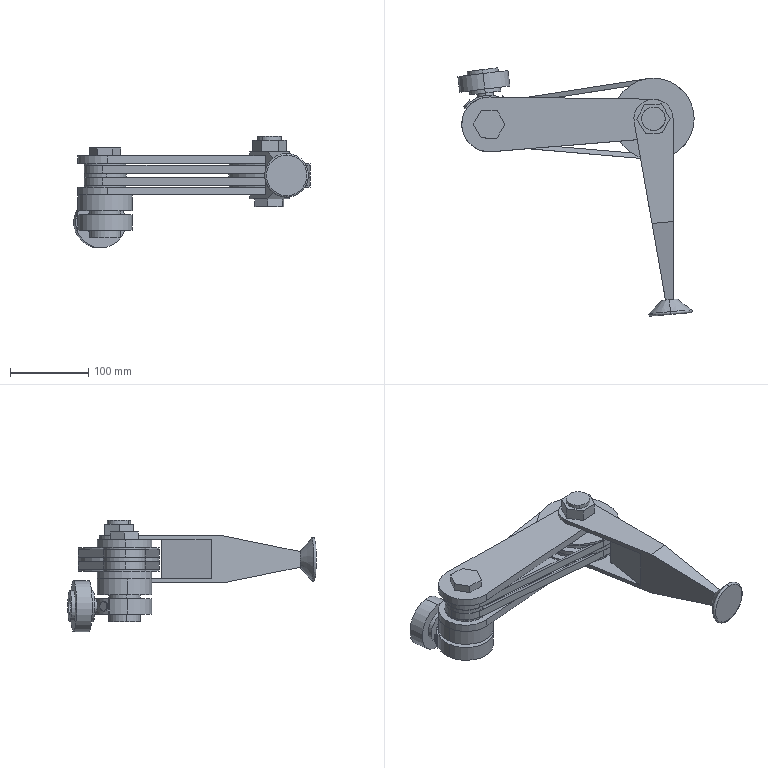Part | SolidWorks | features CompositeCurve 1 | 14 solids | 239 faces | box 302.128 x 317.433 x 142.5 mm | volume 1183356 mm3 | cylinder 107 | plane 104 | cone 18 | spline 8 | torus 2 | commonest cylinder face diameters 30 x20 10 x12 40 x12 70 x8 50 x7 54 x6